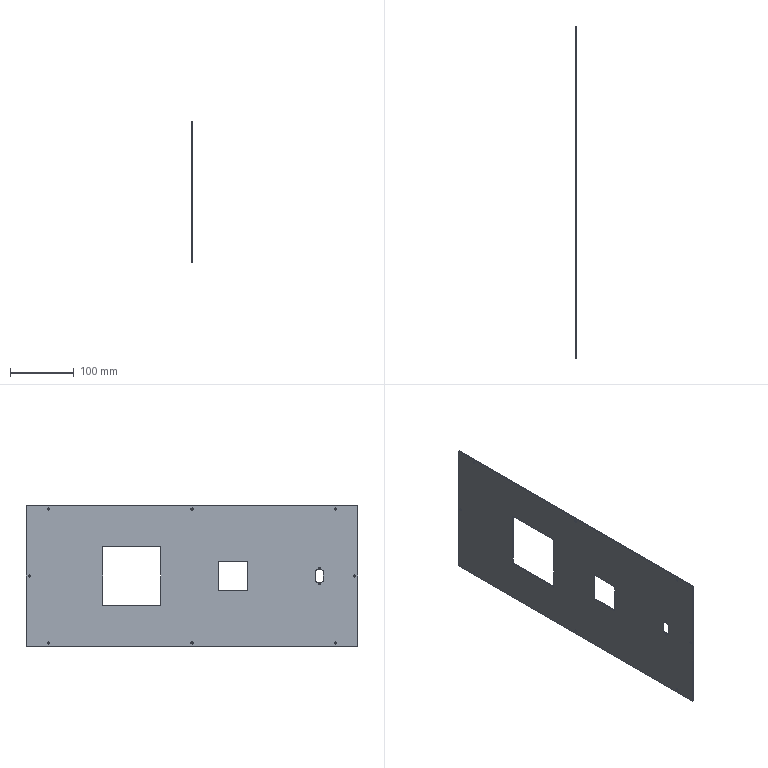Part | STEP file | HESS-408-70-15W-D-11-frame panel | 1 solid | 43 faces | box 1.5 x 520 x 220 mm | volume 155544 mm3 | cylinder 25 | plane 18 | commonest cylinder face diameters 3.2 x16 5 x5 3 x4